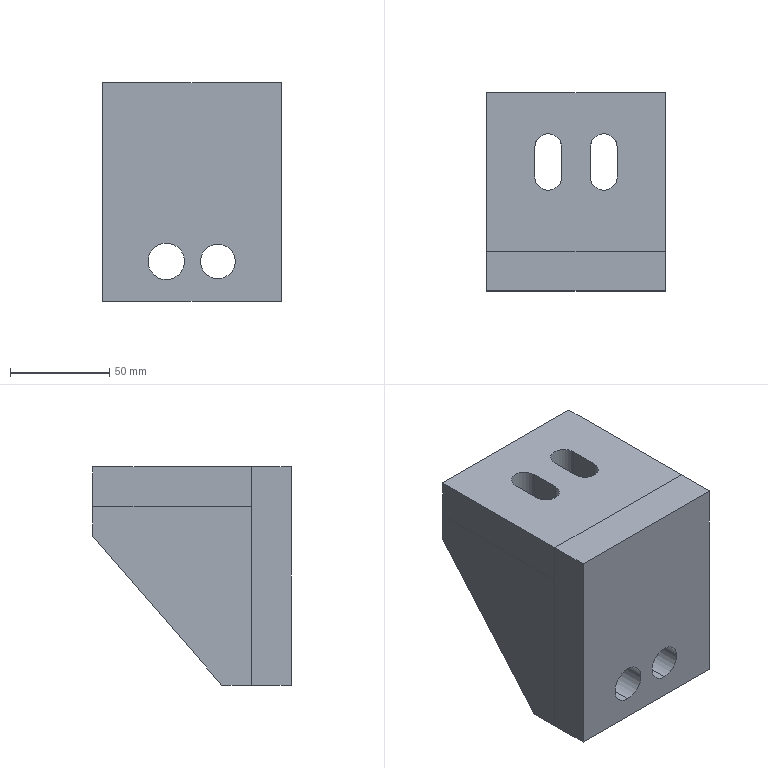Part | SolidWorks | features HoleWzd 3, ICE 2, Extrusion 1, MirrorSolid 1 | 4 solids | 38 faces | box 90 x 100 x 110 mm | volume 460863 mm3 | plane 30 | cylinder 8 | commonest cylinder face diameters 13.5 x4 17.5 x2 18.5 x2
STEP:
#1=CARTESIAN_POINT('',(-45.,20.,35.));
#2=VERTEX_POINT('',#1);
#3=CARTESIAN_POINT('',(-45.,100.,35.));
#4=VERTEX_POINT('',#3);
#5=CARTESIAN_POINT('',(-45.,100.,35.));
#6=DIRECTION('',(0.,1.,0.));
#7=VECTOR('',#6,1000.);
#8=LINE('',#5,#7);
#9=EDGE_CURVE('',#2,#4,#8,.T.);
#10=ORIENTED_EDGE('',*,*,#9,.F.);
#11=CARTESIAN_POINT('',(-30.,20.,35.));
#12=VERTEX_POINT('',#11);
#13=CARTESIAN_POINT('',(-30.,20.,35.));
#14=DIRECTION('',(-1.,0.,0.));
#15=VECTOR('',#14,1000.);
#16=LINE('',#13,#15);
#17=EDGE_CURVE('',#12,#2,#16,.T.);
#18=ORIENTED_EDGE('',*,*,#17,.F.);
#19=CARTESIAN_POINT('',(-30.,100.,35.));
#20=VERTEX_POINT('',#19);
#21=CARTESIAN_POINT('',(-30.,100.,35.));
#22=DIRECTION('',(0.,1.,0.));
#23=VECTOR('',#22,1000.);
#24=LINE('',#21,#23);
#25=EDGE_CURVE('',#12,#20,#24,.T.);
#26=ORIENTED_EDGE('',*,*,#25,.T.);
#27=CARTESIAN_POINT('',(-30.,100.,35.));
#28=DIRECTION('',(-1.,0.,0.));
#29=VECTOR('',#28,1000.);
#30=LINE('',#27,#29);
#31=EDGE_CURVE('',#20,#4,#30,.T.);
#32=ORIENTED_EDGE('',*,*,#31,.T.);
#33=EDGE_LOOP('',(#10,#18,#26,#32));
#34=FACE_OUTER_BOUND('',#33,.T.);
#35=CARTESIAN_POINT('',(-30.,100.,35.));
#36=DIRECTION('',(0.,0.,1.));
#37=DIRECTION('',(1.,0.,0.));
#38=AXIS2_PLACEMENT_3D('',#35,#36,#37);
#39=PLANE('',#38);
#40=ADVANCED_FACE('',(#34),#39,.T.);
#41=CARTESIAN_POINT('',(-45.,20.,-55.));
#42=VERTEX_POINT('',#41);
#43=CARTESIAN_POINT('',(-45.,20.,-55.));
#44=DIRECTION('',(0.,0.,1.));
#45=VECTOR('',#44,1000.);
#46=LINE('',#43,#45);
#47=EDGE_CURVE('',#42,#2,#46,.T.);
#48=ORIENTED_EDGE('',*,*,#47,.F.);
#49=CARTESIAN_POINT('',(-30.,20.,-55.));
#50=VERTEX_POINT('',#49);
#51=CARTESIAN_POINT('',(-30.,20.,-55.));
#52=DIRECTION('',(-1.,0.,0.));
#53=VECTOR('',#52,1000.);
#54=LINE('',#51,#53);
#55=EDGE_CURVE('',#50,#42,#54,.T.);
#56=ORIENTED_EDGE('',*,*,#55,.F.);
#57=CARTESIAN_POINT('',(-30.,20.,-55.));
#58=DIRECTION('',(0.,0.,1.));
#59=VECTOR('',#58,1000.);
#60=LINE('',#57,#59);
#61=EDGE_CURVE('',#50,#12,#60,.T.);
#62=ORIENTED_EDGE('',*,*,#61,.T.);
#63=ORIENTED_EDGE('',*,*,#17,.T.);
#64=EDGE_LOOP('',(#48,#56,#62,#63));
#65=FACE_OUTER_BOUND('',#64,.T.);
#66=CARTESIAN_POINT('',(-30.,20.,-55.));
#67=DIRECTION('',(0.,-1.,0.));
#68=DIRECTION('',(0.,0.,-1.));
#69=AXIS2_PLACEMENT_3D('',#66,#67,#68);
#70=PLANE('',#69);
#71=ADVANCED_FACE('',(#65),#70,.T.);
#72=CARTESIAN_POINT('',(-45.,35.,-55.));
#73=VERTEX_POINT('',#72);
#74=CARTESIAN_POINT('',(-45.,35.,-55.));
#75=DIRECTION('',(0.,-1.,0.));
#76=VECTOR('',#75,1000.);
#77=LINE('',#74,#76);
#78=EDGE_CURVE('',#73,#42,#77,.T.);
#79=ORIENTED_EDGE('',*,*,#78,.F.);
#80=CARTESIAN_POINT('',(-30.,35.,-55.));
#81=VERTEX_POINT('',#80);
#82=CARTESIAN_POINT('',(-30.,35.,-55.));
#83=DIRECTION('',(-1.,0.,0.));
#84=VECTOR('',#83,1000.);
#85=LINE('',#82,#84);
#86=EDGE_CURVE('',#81,#73,#85,.T.);
#87=ORIENTED_EDGE('',*,*,#86,.F.);
#88=CARTESIAN_POINT('',(-30.,35.,-55.));
#89=DIRECTION('',(0.,-1.,0.));
#90=VECTOR('',#89,1000.);
#91=LINE('',#88,#90);
#92=EDGE_CURVE('',#81,#50,#91,.T.);
#93=ORIENTED_EDGE('',*,*,#92,.T.);
#94=ORIENTED_EDGE('',*,*,#55,.T.);
#95=EDGE_LOOP('',(#79,#87,#93,#94));
#96=FACE_OUTER_BOUND('',#95,.T.);
#97=CARTESIAN_POINT('',(-30.,35.,-55.));
#98=DIRECTION('',(0.,0.,-1.));
#99=DIRECTION('',(-1.,0.,0.));
#100=AXIS2_PLACEMENT_3D('',#97,#98,#99);
#101=PLANE('',#100);
#102=ADVANCED_FACE('',(#96),#101,.T.);
#103=CARTESIAN_POINT('',(-45.,100.,20.));
#104=VERTEX_POINT('',#103);
#105=CARTESIAN_POINT('',(-45.,100.,20.));
#106=DIRECTION('',(0.,-0.6549,-0.7557));
#107=VECTOR('',#106,1000.);
#108=LINE('',#105,#107);
#109=EDGE_CURVE('',#104,#73,#108,.T.);
#110=ORIENTED_EDGE('',*,*,#109,.F.);
#111=CARTESIAN_POINT('',(-30.,100.,20.));
#112=VERTEX_POINT('',#111);
#113=CARTESIAN_POINT('',(-30.,100.,20.));
#114=DIRECTION('',(-1.,0.,0.));
#115=VECTOR('',#114,1000.);
#116=LINE('',#113,#115);
#117=EDGE_CURVE('',#112,#104,#116,.T.);
#118=ORIENTED_EDGE('',*,*,#117,.F.);
#119=CARTESIAN_POINT('',(-30.,100.,20.));
#120=DIRECTION('',(0.,-0.6549,-0.7557));
#121=VECTOR('',#120,1000.);
#122=LINE('',#119,#121);
#123=EDGE_CURVE('',#112,#81,#122,.T.);
#124=ORIENTED_EDGE('',*,*,#123,.T.);
#125=ORIENTED_EDGE('',*,*,#86,.T.);
#126=EDGE_LOOP('',(#110,#118,#124,#125));
#127=FACE_OUTER_BOUND('',#126,.T.);
#128=CARTESIAN_POINT('',(-30.,100.,20.));
#129=DIRECTION('',(0.,0.7557,-0.6549));
#130=DIRECTION('',(0.,0.6549,0.7557));
#131=AXIS2_PLACEMENT_3D('',#128,#129,#130);
#132=PLANE('',#131);
#133=ADVANCED_FACE('',(#127),#132,.T.);
#134=CARTESIAN_POINT('',(-45.,100.,35.));
#135=DIRECTION('',(0.,0.,-1.));
#136=VECTOR('',#135,1000.);
#137=LINE('',#134,#136);
#138=EDGE_CURVE('',#4,#104,#137,.T.);
#139=ORIENTED_EDGE('',*,*,#138,.F.);
#140=ORIENTED_EDGE('',*,*,#31,.F.);
#141=CARTESIAN_POINT('',(-30.,100.,35.));
#142=DIRECTION('',(0.,0.,-1.));
#143=VECTOR('',#142,1000.);
#144=LINE('',#141,#143);
#145=EDGE_CURVE('',#20,#112,#144,.T.);
#146=ORIENTED_EDGE('',*,*,#145,.T.);
#147=ORIENTED_EDGE('',*,*,#117,.T.);
#148=EDGE_LOOP('',(#139,#140,#146,#147));
#149=FACE_OUTER_BOUND('',#148,.T.);
#150=CARTESIAN_POINT('',(-30.,100.,35.));
#151=DIRECTION('',(0.,1.,0.));
#152=DIRECTION('',(0.,0.,1.));
#153=AXIS2_PLACEMENT_3D('',#150,#151,#152);
#154=PLANE('',#153);
#155=ADVANCED_FACE('',(#149),#154,.T.);
#156=ORIENTED_EDGE('',*,*,#25,.F.);
#157=ORIENTED_EDGE('',*,*,#61,.F.);
#158=ORIENTED_EDGE('',*,*,#92,.F.);
#159=ORIENTED_EDGE('',*,*,#123,.F.);
#160=ORIENTED_EDGE('',*,*,#145,.F.);
#161=EDGE_LOOP('',(#156,#157,#158,#159,#160));
#162=FACE_OUTER_BOUND('',#161,.T.);
#163=CARTESIAN_POINT('',(-30.,0.,0.));
#164=DIRECTION('',(-1.,0.,0.));
#165=DIRECTION('',(0.,0.,1.));
#166=AXIS2_PLACEMENT_3D('',#163,#164,#165);
#167=PLANE('',#166);
#168=ADVANCED_FACE('',(#162),#167,.F.);
#169=ORIENTED_EDGE('',*,*,#9,.T.);
#170=ORIENTED_EDGE('',*,*,#138,.T.);
#171=ORIENTED_EDGE('',*,*,#109,.T.);
#172=ORIENTED_EDGE('',*,*,#78,.T.);
#173=ORIENTED_EDGE('',*,*,#47,.T.);
#174=EDGE_LOOP('',(#169,#170,#171,#172,#173));
#175=FACE_OUTER_BOUND('',#174,.T.);
#176=CARTESIAN_POINT('',(-45.,0.,0.));
#177=DIRECTION('',(-1.,0.,0.));
#178=DIRECTION('',(0.,0.,1.));
#179=AXIS2_PLACEMENT_3D('',#176,#177,#178);
#180=PLANE('',#179);
#181=ADVANCED_FACE('',(#175),#180,.T.);
#182=CLOSED_SHELL('',(#40,#71,#102,#133,#155,#168,#181));
#183=MANIFOLD_SOLID_BREP('',#182);
#184=CARTESIAN_POINT('',(45.,20.,35.));
#185=VERTEX_POINT('',#184);
#186=CARTESIAN_POINT('',(45.,100.,35.));
#187=VERTEX_POINT('',#186);
#188=CARTESIAN_POINT('',(45.,100.,35.));
#189=DIRECTION('',(0.,1.,0.));
#190=VECTOR('',#189,1000.);
#191=LINE('',#188,#190);
#192=EDGE_CURVE('',#185,#187,#191,.T.);
#193=ORIENTED_EDGE('',*,*,#192,.T.);
#194=CARTESIAN_POINT('',(30.,100.,35.));
#195=VERTEX_POINT('',#194);
#196=CARTESIAN_POINT('',(30.,100.,35.));
#197=DIRECTION('',(1.,0.,0.));
#198=VECTOR('',#197,1000.);
#199=LINE('',#196,#198);
#200=EDGE_CURVE('',#195,#187,#199,.T.);
#201=ORIENTED_EDGE('',*,*,#200,.F.);
#202=CARTESIAN_POINT('',(30.,20.,35.));
#203=VERTEX_POINT('',#202);
#204=CARTESIAN_POINT('',(30.,100.,35.));
#205=DIRECTION('',(0.,1.,0.));
#206=VECTOR('',#205,1000.);
#207=LINE('',#204,#206);
#208=EDGE_CURVE('',#203,#195,#207,.T.);
#209=ORIENTED_EDGE('',*,*,#208,.F.);
#210=CARTESIAN_POINT('',(30.,20.,35.));
#211=DIRECTION('',(1.,0.,0.));
#212=VECTOR('',#211,1000.);
#213=LINE('',#210,#212);
#214=EDGE_CURVE('',#203,#185,#213,.T.);
#215=ORIENTED_EDGE('',*,*,#214,.T.);
#216=EDGE_LOOP('',(#193,#201,#209,#215));
#217=FACE_OUTER_BOUND('',#216,.T.);
#218=CARTESIAN_POINT('',(30.,100.,35.));
#219=DIRECTION('',(0.,0.,1.));
#220=DIRECTION('',(-1.,0.,0.));
#221=AXIS2_PLACEMENT_3D('',#218,#219,#220);
#222=PLANE('',#221);
#223=ADVANCED_FACE('',(#217),#222,.T.);
#224=CARTESIAN_POINT('',(45.,20.,-55.));
#225=VERTEX_POINT('',#224);
#226=CARTESIAN_POINT('',(45.,20.,-55.));
#227=DIRECTION('',(0.,0.,1.));
#228=VECTOR('',#227,1000.);
#229=LINE('',#226,#228);
#230=EDGE_CURVE('',#225,#185,#229,.T.);
#231=ORIENTED_EDGE('',*,*,#230,.T.);
#232=ORIENTED_EDGE('',*,*,#214,.F.);
#233=CARTESIAN_POINT('',(30.,20.,-55.));
#234=VERTEX_POINT('',#233);
#235=CARTESIAN_POINT('',(30.,20.,-55.));
#236=DIRECTION('',(0.,0.,1.));
#237=VECTOR('',#236,1000.);
#238=LINE('',#235,#237);
#239=EDGE_CURVE('',#234,#203,#238,.T.);
#240=ORIENTED_EDGE('',*,*,#239,.F.);
#241=CARTESIAN_POINT('',(30.,20.,-55.));
#242=DIRECTION('',(1.,0.,0.));
#243=VECTOR('',#242,1000.);
#244=LINE('',#241,#243);
#245=EDGE_CURVE('',#234,#225,#244,.T.);
#246=ORIENTED_EDGE('',*,*,#245,.T.);
#247=EDGE_LOOP('',(#231,#232,#240,#246));
#248=FACE_OUTER_BOUND('',#247,.T.);
#249=CARTESIAN_POINT('',(30.,20.,-55.));
#250=DIRECTION('',(0.,-1.,0.));
#251=DIRECTION('',(0.,0.,-1.));
#252=AXIS2_PLACEMENT_3D('',#249,#250,#251);
#253=PLANE('',#252);
#254=ADVANCED_FACE('',(#248),#253,.T.);
#255=CARTESIAN_POINT('',(45.,35.,-55.));
#256=VERTEX_POINT('',#255);
#257=CARTESIAN_POINT('',(45.,35.,-55.));
#258=DIRECTION('',(0.,-1.,0.));
#259=VECTOR('',#258,1000.);
#260=LINE('',#257,#259);
#261=EDGE_CURVE('',#256,#225,#260,.T.);
#262=ORIENTED_EDGE('',*,*,#261,.T.);
#263=ORIENTED_EDGE('',*,*,#245,.F.);
#264=CARTESIAN_POINT('',(30.,35.,-55.));
#265=VERTEX_POINT('',#264);
#266=CARTESIAN_POINT('',(30.,35.,-55.));
#267=DIRECTION('',(0.,-1.,0.));
#268=VECTOR('',#267,1000.);
#269=LINE('',#266,#268);
#270=EDGE_CURVE('',#265,#234,#269,.T.);
#271=ORIENTED_EDGE('',*,*,#270,.F.);
#272=CARTESIAN_POINT('',(30.,35.,-55.));
#273=DIRECTION('',(1.,0.,0.));
#274=VECTOR('',#273,1000.);
#275=LINE('',#272,#274);
#276=EDGE_CURVE('',#265,#256,#275,.T.);
#277=ORIENTED_EDGE('',*,*,#276,.T.);
#278=EDGE_LOOP('',(#262,#263,#271,#277));
#279=FACE_OUTER_BOUND('',#278,.T.);
#280=CARTESIAN_POINT('',(30.,35.,-55.));
#281=DIRECTION('',(0.,0.,-1.));
#282=DIRECTION('',(1.,0.,0.));
#283=AXIS2_PLACEMENT_3D('',#280,#281,#282);
#284=PLANE('',#283);
#285=ADVANCED_FACE('',(#279),#284,.T.);
#286=CARTESIAN_POINT('',(45.,100.,20.));
#287=VERTEX_POINT('',#286);
#288=CARTESIAN_POINT('',(45.,100.,20.));
#289=DIRECTION('',(0.,-0.6549,-0.7557));
#290=VECTOR('',#289,1000.);
#291=LINE('',#288,#290);
#292=EDGE_CURVE('',#287,#256,#291,.T.);
#293=ORIENTED_EDGE('',*,*,#292,.T.);
#294=ORIENTED_EDGE('',*,*,#276,.F.);
#295=CARTESIAN_POINT('',(30.,100.,20.));
#296=VERTEX_POINT('',#295);
#297=CARTESIAN_POINT('',(30.,100.,20.));
#298=DIRECTION('',(0.,-0.6549,-0.7557));
#299=VECTOR('',#298,1000.);
#300=LINE('',#297,#299);
#301=EDGE_CURVE('',#296,#265,#300,.T.);
#302=ORIENTED_EDGE('',*,*,#301,.F.);
#303=CARTESIAN_POINT('',(30.,100.,20.));
#304=DIRECTION('',(1.,0.,0.));
#305=VECTOR('',#304,1000.);
#306=LINE('',#303,#305);
#307=EDGE_CURVE('',#296,#287,#306,.T.);
#308=ORIENTED_EDGE('',*,*,#307,.T.);
#309=EDGE_LOOP('',(#293,#294,#302,#308));
#310=FACE_OUTER_BOUND('',#309,.T.);
#311=CARTESIAN_POINT('',(30.,100.,20.));
#312=DIRECTION('',(0.,0.7557,-0.6549));
#313=DIRECTION('',(0.,0.6549,0.7557));
#314=AXIS2_PLACEMENT_3D('',#311,#312,#313);
#315=PLANE('',#314);
#316=ADVANCED_FACE('',(#310),#315,.T.);
#317=CARTESIAN_POINT('',(45.,100.,35.));
#318=DIRECTION('',(0.,0.,-1.));
#319=VECTOR('',#318,1000.);
#320=LINE('',#317,#319);
#321=EDGE_CURVE('',#187,#287,#320,.T.);
#322=ORIENTED_EDGE('',*,*,#321,.T.);
#323=ORIENTED_EDGE('',*,*,#307,.F.);
#324=CARTESIAN_POINT('',(30.,100.,35.));
#325=DIRECTION('',(0.,0.,-1.));
#326=VECTOR('',#325,1000.);
#327=LINE('',#324,#326);
#328=EDGE_CURVE('',#195,#296,#327,.T.);
#329=ORIENTED_EDGE('',*,*,#328,.F.);
#330=ORIENTED_EDGE('',*,*,#200,.T.);
#331=EDGE_LOOP('',(#322,#323,#329,#330));
#332=FACE_OUTER_BOUND('',#331,.T.);
#333=CARTESIAN_POINT('',(30.,100.,35.));
#334=DIRECTION('',(0.,1.,0.));
#335=DIRECTION('',(0.,0.,1.));
#336=AXIS2_PLACEMENT_3D('',#333,#334,#335);
#337=PLANE('',#336);
#338=ADVANCED_FACE('',(#332),#337,.T.);
#339=ORIENTED_EDGE('',*,*,#208,.T.);
#340=ORIENTED_EDGE('',*,*,#328,.T.);
#341=ORIENTED_EDGE('',*,*,#301,.T.);
#342=ORIENTED_EDGE('',*,*,#270,.T.);
#343=ORIENTED_EDGE('',*,*,#239,.T.);
#344=EDGE_LOOP('',(#339,#340,#341,#342,#343));
#345=FACE_OUTER_BOUND('',#344,.T.);
#346=CARTESIAN_POINT('',(30.,0.,0.));
#347=DIRECTION('',(1.,0.,0.));
#348=DIRECTION('',(0.,0.,1.));
#349=AXIS2_PLACEMENT_3D('',#346,#347,#348);
#350=PLANE('',#349);
#351=ADVANCED_FACE('',(#345),#350,.F.);
#352=ORIENTED_EDGE('',*,*,#192,.F.);
#353=ORIENTED_EDGE('',*,*,#230,.F.);
#354=ORIENTED_EDGE('',*,*,#261,.F.);
#355=ORIENTED_EDGE('',*,*,#292,.F.);
#356=ORIENTED_EDGE('',*,*,#321,.F.);
#357=EDGE_LOOP('',(#352,#353,#354,#355,#356));
#358=FACE_OUTER_BOUND('',#357,.T.);
#359=CARTESIAN_POINT('',(45.,0.,0.));
#360=DIRECTION('',(1.,0.,0.));
#361=DIRECTION('',(0.,0.,1.));
#362=AXIS2_PLACEMENT_3D('',#359,#360,#361);
#363=PLANE('',#362);
#364=ADVANCED_FACE('',(#358),#363,.T.);
#365=CLOSED_SHELL('',(#223,#254,#285,#316,#338,#351,#364));
#366=MANIFOLD_SOLID_BREP('',#365);
#367=CARTESIAN_POINT('',(-45.,20.,35.));
#368=VERTEX_POINT('',#367);
#369=CARTESIAN_POINT('',(-45.,20.,55.));
#370=VERTEX_POINT('',#369);
#371=CARTESIAN_POINT('',(-45.,20.,55.));
#372=DIRECTION('',(0.,0.,1.));
#373=VECTOR('',#372,1000.);
#374=LINE('',#371,#373);
#375=EDGE_CURVE('',#368,#370,#374,.T.);
#376=ORIENTED_EDGE('',*,*,#375,.T.);
#377=CARTESIAN_POINT('',(-45.,100.,55.));
#378=VERTEX_POINT('',#377);
#379=CARTESIAN_POINT('',(-45.,100.,55.));
#380=DIRECTION('',(0.,-1.,0.));
#381=VECTOR('',#380,1000.);
#382=LINE('',#379,#381);
#383=EDGE_CURVE('',#378,#370,#382,.T.);
#384=ORIENTED_EDGE('',*,*,#383,.F.);
#385=CARTESIAN_POINT('',(-45.,100.,35.));
#386=VERTEX_POINT('',#385);
#387=CARTESIAN_POINT('',(-45.,100.,55.));
#388=DIRECTION('',(0.,0.,1.));
#389=VECTOR('',#388,1000.);
#390=LINE('',#387,#389);
#391=EDGE_CURVE('',#386,#378,#390,.T.);
#392=ORIENTED_EDGE('',*,*,#391,.F.);
#393=CARTESIAN_POINT('',(-45.,100.,35.));
#394=DIRECTION('',(0.,-1.,0.));
#395=VECTOR('',#394,1000.);
#396=LINE('',#393,#395);
#397=EDGE_CURVE('',#386,#368,#396,.T.);
#398=ORIENTED_EDGE('',*,*,#397,.T.);
#399=EDGE_LOOP('',(#376,#384,#392,#398));
#400=FACE_OUTER_BOUND('',#399,.T.);
#401=CARTESIAN_POINT('',(-45.,100.,55.));
#402=DIRECTION('',(1.,0.,0.));
#403=DIRECTION('',(0.,0.,-1.));
#404=AXIS2_PLACEMENT_3D('',#401,#402,#403);
#405=PLANE('',#404);
#406=ADVANCED_FACE('',(#400),#405,.F.);
#407=CARTESIAN_POINT('',(20.75,72.5,55.));
#408=VERTEX_POINT('',#407);
#409=CARTESIAN_POINT('',(20.75,57.5,55.));
#410=VERTEX_POINT('',#409);
#411=CARTESIAN_POINT('',(20.75,72.5,55.));
#412=DIRECTION('',(0.,-1.,0.));
#413=VECTOR('',#412,1000.);
#414=LINE('',#411,#413);
#415=EDGE_CURVE('',#408,#410,#414,.T.);
#416=ORIENTED_EDGE('',*,*,#415,.T.);
#417=CARTESIAN_POINT('',(7.25,57.5,55.));
#418=VERTEX_POINT('',#417);
#419=CARTESIAN_POINT('',(14.,57.5,55.));
#420=DIRECTION('',(0.,0.,-1.));
#421=DIRECTION('',(-1.,0.,0.));
#422=AXIS2_PLACEMENT_3D('',#419,#420,#421);
#423=CIRCLE('',#422,6.75);
#424=EDGE_CURVE('',#410,#418,#423,.T.);
#425=ORIENTED_EDGE('',*,*,#424,.T.);
#426=CARTESIAN_POINT('',(7.25,72.5,55.));
#427=VERTEX_POINT('',#426);
#428=CARTESIAN_POINT('',(7.25,72.5,55.));
#429=DIRECTION('',(0.,-1.,0.));
#430=VECTOR('',#429,1000.);
#431=LINE('',#428,#430);
#432=EDGE_CURVE('',#427,#418,#431,.T.);
#433=ORIENTED_EDGE('',*,*,#432,.F.);
#434=CARTESIAN_POINT('',(14.,72.5,55.));
#435=DIRECTION('',(0.,0.,-1.));
#436=DIRECTION('',(-1.,0.,0.));
#437=AXIS2_PLACEMENT_3D('',#434,#435,#436);
#438=CIRCLE('',#437,6.75);
#439=EDGE_CURVE('',#427,#408,#438,.T.);
#440=ORIENTED_EDGE('',*,*,#439,.T.);
#441=EDGE_LOOP('',(#416,#425,#433,#440));
#442=FACE_BOUND('',#441,.T.);
#443=CARTESIAN_POINT('',(-20.75,72.5,55.));
#444=VERTEX_POINT('',#443);
#445=CARTESIAN_POINT('',(-7.25,72.5,55.));
#446=VERTEX_POINT('',#445);
#447=CARTESIAN_POINT('',(-14.,72.5,55.));
#448=DIRECTION('',(0.,0.,-1.));
#449=DIRECTION('',(-1.,0.,0.));
#450=AXIS2_PLACEMENT_3D('',#447,#448,#449);
#451=CIRCLE('',#450,6.75);
#452=EDGE_CURVE('',#444,#446,#451,.T.);
#453=ORIENTED_EDGE('',*,*,#452,.T.);
#454=CARTESIAN_POINT('',(-7.25,57.5,55.));
#455=VERTEX_POINT('',#454);
#456=CARTESIAN_POINT('',(-7.25,72.5,55.));
#457=DIRECTION('',(0.,-1.,0.));
#458=VECTOR('',#457,1000.);
#459=LINE('',#456,#458);
#460=EDGE_CURVE('',#446,#455,#459,.T.);
#461=ORIENTED_EDGE('',*,*,#460,.T.);
#462=CARTESIAN_POINT('',(-20.75,57.5,55.));
#463=VERTEX_POINT('',#462);
#464=CARTESIAN_POINT('',(-14.,57.5,55.));
#465=DIRECTION('',(0.,0.,-1.));
#466=DIRECTION('',(-1.,0.,0.));
#467=AXIS2_PLACEMENT_3D('',#464,#465,#466);
#468=CIRCLE('',#467,6.75);
#469=EDGE_CURVE('',#455,#463,#468,.T.);
#470=ORIENTED_EDGE('',*,*,#469,.T.);
#471=CARTESIAN_POINT('',(-20.75,72.5,55.));
#472=DIRECTION('',(0.,-1.,0.));
#473=VECTOR('',#472,1000.);
#474=LINE('',#471,#473);
#475=EDGE_CURVE('',#444,#463,#474,.T.);
#476=ORIENTED_EDGE('',*,*,#475,.F.);
#477=EDGE_LOOP('',(#453,#461,#470,#476));
#478=FACE_BOUND('',#477,.T.);
#479=CARTESIAN_POINT('',(45.,20.,55.));
#480=VERTEX_POINT('',#479);
#481=CARTESIAN_POINT('',(-45.,20.,55.));
#482=DIRECTION('',(1.,0.,0.));
#483=VECTOR('',#482,1000.);
#484=LINE('',#481,#483);
#485=EDGE_CURVE('',#370,#480,#484,.T.);
#486=ORIENTED_EDGE('',*,*,#485,.T.);
#487=CARTESIAN_POINT('',(45.,100.,55.));
#488=VERTEX_POINT('',#487);
#489=CARTESIAN_POINT('',(45.,100.,55.));
#490=DIRECTION('',(0.,-1.,0.));
#491=VECTOR('',#490,1000.);
#492=LINE('',#489,#491);
#493=EDGE_CURVE('',#488,#480,#492,.T.);
#494=ORIENTED_EDGE('',*,*,#493,.F.);
#495=CARTESIAN_POINT('',(-45.,100.,55.));
#496=DIRECTION('',(1.,0.,0.));
#497=VECTOR('',#496,1000.);
#498=LINE('',#495,#497);
#499=EDGE_CURVE('',#378,#488,#498,.T.);
#500=ORIENTED_EDGE('',*,*,#499,.F.);
#501=ORIENTED_EDGE('',*,*,#383,.T.);
#502=EDGE_LOOP('',(#486,#494,#500,#501));
#503=FACE_OUTER_BOUND('',#502,.T.);
#504=CARTESIAN_POINT('',(-45.,100.,55.));
#505=DIRECTION('',(0.,0.,-1.));
#506=DIRECTION('',(-1.,0.,0.));
#507=AXIS2_PLACEMENT_3D('',#504,#505,#506);
#508=PLANE('',#507);
#509=ADVANCED_FACE('',(#442,#478,#503),#508,.F.);
#510=CARTESIAN_POINT('',(45.,20.,35.));
#511=VERTEX_POINT('',#510);
#512=CARTESIAN_POINT('',(45.,20.,55.));
#513=DIRECTION('',(0.,0.,-1.));
#514=VECTOR('',#513,1000.);
#515=LINE('',#512,#514);
#516=EDGE_CURVE('',#480,#511,#515,.T.);
#517=ORIENTED_EDGE('',*,*,#516,.T.);
#518=CARTESIAN_POINT('',(45.,100.,35.));
#519=VERTEX_POINT('',#518);
#520=CARTESIAN_POINT('',(45.,100.,35.));
#521=DIRECTION('',(0.,-1.,0.));
#522=VECTOR('',#521,1000.);
#523=LINE('',#520,#522);
#524=EDGE_CURVE('',#519,#511,#523,.T.);
#525=ORIENTED_EDGE('',*,*,#524,.F.);
#526=CARTESIAN_POINT('',(45.,100.,55.));
#527=DIRECTION('',(0.,0.,-1.));
#528=VECTOR('',#527,1000.);
#529=LINE('',#526,#528);
#530=EDGE_CURVE('',#488,#519,#529,.T.);
#531=ORIENTED_EDGE('',*,*,#530,.F.);
#532=ORIENTED_EDGE('',*,*,#493,.T.);
#533=EDGE_LOOP('',(#517,#525,#531,#532));
#534=FACE_OUTER_BOUND('',#533,.T.);
#535=CARTESIAN_POINT('',(45.,100.,55.));
#536=DIRECTION('',(-1.,0.,0.));
#537=DIRECTION('',(0.,0.,1.));
#538=AXIS2_PLACEMENT_3D('',#535,#536,#537);
#539=PLANE('',#538);
#540=ADVANCED_FACE('',(#534),#539,.F.);
#541=CARTESIAN_POINT('',(20.75,57.5,35.));
#542=VERTEX_POINT('',#541);
#543=CARTESIAN_POINT('',(7.25,57.5,35.));
#544=VERTEX_POINT('',#543);
#545=CARTESIAN_POINT('',(14.,57.5,35.));
#546=DIRECTION('',(0.,0.,-1.));
#547=DIRECTION('',(-1.,0.,0.));
#548=AXIS2_PLACEMENT_3D('',#545,#546,#547);
#549=CIRCLE('',#548,6.75);
#550=EDGE_CURVE('',#542,#544,#549,.T.);
#551=ORIENTED_EDGE('',*,*,#550,.F.);
#552=CARTESIAN_POINT('',(20.75,72.5,35.));
#553=VERTEX_POINT('',#552);
#554=CARTESIAN_POINT('',(20.75,72.5,35.));
#555=DIRECTION('',(0.,-1.,0.));
#556=VECTOR('',#555,1000.);
#557=LINE('',#554,#556);
#558=EDGE_CURVE('',#553,#542,#557,.T.);
#559=ORIENTED_EDGE('',*,*,#558,.F.);
#560=CARTESIAN_POINT('',(7.25,72.5,35.));
#561=VERTEX_POINT('',#560);
#562=CARTESIAN_POINT('',(14.,72.5,35.));
#563=DIRECTION('',(0.,0.,-1.));
#564=DIRECTION('',(-1.,0.,0.));
#565=AXIS2_PLACEMENT_3D('',#562,#563,#564);
#566=CIRCLE('',#565,6.75);
#567=EDGE_CURVE('',#561,#553,#566,.T.);
#568=ORIENTED_EDGE('',*,*,#567,.F.);
#569=CARTESIAN_POINT('',(7.25,72.5,35.));
#570=DIRECTION('',(0.,-1.,0.));
#571=VECTOR('',#570,1000.);
#572=LINE('',#569,#571);
#573=EDGE_CURVE('',#561,#544,#572,.T.);
#574=ORIENTED_EDGE('',*,*,#573,.T.);
#575=EDGE_LOOP('',(#551,#559,#568,#574));
#576=FACE_BOUND('',#575,.T.);
#577=CARTESIAN_POINT('',(-20.75,72.5,35.));
#578=VERTEX_POINT('',#577);
#579=CARTESIAN_POINT('',(-7.25,72.5,35.));
#580=VERTEX_POINT('',#579);
#581=CARTESIAN_POINT('',(-14.,72.5,35.));
#582=DIRECTION('',(0.,0.,-1.));
#583=DIRECTION('',(-1.,0.,0.));
#584=AXIS2_PLACEMENT_3D('',#581,#582,#583);
#585=CIRCLE('',#584,6.75);
#586=EDGE_CURVE('',#578,#580,#585,.T.);
#587=ORIENTED_EDGE('',*,*,#586,.F.);
#588=CARTESIAN_POINT('',(-20.75,57.5,35.));
#589=VERTEX_POINT('',#588);
#590=CARTESIAN_POINT('',(-20.75,72.5,35.));
#591=DIRECTION('',(0.,-1.,0.));
#592=VECTOR('',#591,1000.);
#593=LINE('',#590,#592);
#594=EDGE_CURVE('',#578,#589,#593,.T.);
#595=ORIENTED_EDGE('',*,*,#594,.T.);
#596=CARTESIAN_POINT('',(-7.25,57.5,35.));
#597=VERTEX_POINT('',#596);
#598=CARTESIAN_POINT('',(-14.,57.5,35.));
#599=DIRECTION('',(0.,0.,-1.));
#600=DIRECTION('',(-1.,0.,0.));
#601=AXIS2_PLACEMENT_3D('',#598,#599,#600);
#602=CIRCLE('',#601,6.75);
#603=EDGE_CURVE('',#597,#589,#602,.T.);
#604=ORIENTED_EDGE('',*,*,#603,.F.);
#605=CARTESIAN_POINT('',(-7.25,72.5,35.));
#606=DIRECTION('',(0.,-1.,0.));
#607=VECTOR('',#606,1000.);
#608=LINE('',#605,#607);
#609=EDGE_CURVE('',#580,#597,#608,.T.);
#610=ORIENTED_EDGE('',*,*,#609,.F.);
#611=EDGE_LOOP('',(#587,#595,#604,#610));
#612=FACE_BOUND('',#611,.T.);
#613=CARTESIAN_POINT('',(-45.,20.,35.));
#614=DIRECTION('',(-1.,0.,0.));
#615=VECTOR('',#614,1000.);
#616=LINE('',#613,#615);
#617=EDGE_CURVE('',#511,#368,#616,.T.);
#618=ORIENTED_EDGE('',*,*,#617,.T.);
#619=ORIENTED_EDGE('',*,*,#397,.F.);
#620=CARTESIAN_POINT('',(-45.,100.,35.));
#621=DIRECTION('',(-1.,0.,0.));
#622=VECTOR('',#621,1000.);
#623=LINE('',#620,#622);
#624=EDGE_CURVE('',#519,#386,#623,.T.);
#625=ORIENTED_EDGE('',*,*,#624,.F.);
#626=ORIENTED_EDGE('',*,*,#524,.T.);
#627=EDGE_LOOP('',(#618,#619,#625,#626));
#628=FACE_OUTER_BOUND('',#627,.T.);
#629=CARTESIAN_POINT('',(-45.,100.,35.));
#630=DIRECTION('',(0.,0.,1.));
#631=DIRECTION('',(1.,0.,0.));
#632=AXIS2_PLACEMENT_3D('',#629,#630,#631);
#633=PLANE('',#632);
#634=ADVANCED_FACE('',(#576,#612,#628),#633,.F.);
#635=ORIENTED_EDGE('',*,*,#391,.T.);
#636=ORIENTED_EDGE('',*,*,#499,.T.);
#637=ORIENTED_EDGE('',*,*,#530,.T.);
#638=ORIENTED_EDGE('',*,*,#624,.T.);
#639=EDGE_LOOP('',(#635,#636,#637,#638));
#640=FACE_OUTER_BOUND('',#639,.T.);
#641=CARTESIAN_POINT('',(0.,100.,0.));
#642=DIRECTION('',(0.,-1.,0.));
#643=DIRECTION('',(0.,0.,-1.));
#644=AXIS2_PLACEMENT_3D('',#641,#642,#643);
#645=PLANE('',#644);
#646=ADVANCED_FACE('',(#640),#645,.F.);
#647=ORIENTED_EDGE('',*,*,#375,.F.);
#648=ORIENTED_EDGE('',*,*,#617,.F.);
#649=ORIENTED_EDGE('',*,*,#516,.F.);
#650=ORIENTED_EDGE('',*,*,#485,.F.);
#651=EDGE_LOOP('',(#647,#648,#649,#650));
#652=FACE_OUTER_BOUND('',#651,.T.);
#653=CARTESIAN_POINT('',(0.,20.,0.));
#654=DIRECTION('',(0.,-1.,0.));
#655=DIRECTION('',(0.,0.,-1.));
#656=AXIS2_PLACEMENT_3D('',#653,#654,#655);
#657=PLANE('',#656);
#658=ADVANCED_FACE('',(#652),#657,.T.);
#659=ORIENTED_EDGE('',*,*,#469,.F.);
#660=CARTESIAN_POINT('',(-7.25,57.5,55.));
#661=DIRECTION('',(0.,0.,1.));
#662=VECTOR('',#661,1000.);
#663=LINE('',#660,#662);
#664=EDGE_CURVE('',#597,#455,#663,.T.);
#665=ORIENTED_EDGE('',*,*,#664,.F.);
#666=ORIENTED_EDGE('',*,*,#603,.T.);
#667=CARTESIAN_POINT('',(-20.75,57.5,35.));
#668=DIRECTION('',(0.,0.,-1.));
#669=VECTOR('',#668,1000.);
#670=LINE('',#667,#669);
#671=EDGE_CURVE('',#463,#589,#670,.T.);
#672=ORIENTED_EDGE('',*,*,#671,.F.);
#673=EDGE_LOOP('',(#659,#665,#666,#672));
#674=FACE_OUTER_BOUND('',#673,.T.);
#675=CARTESIAN_POINT('',(-14.,57.5,35.));
#676=DIRECTION('',(0.,0.,-1.));
#677=DIRECTION('',(-1.,0.,0.));
#678=AXIS2_PLACEMENT_3D('',#675,#676,#677);
#679=CYLINDRICAL_SURFACE('',#678,6.75);
#680=ADVANCED_FACE('',(#674),#679,.F.);
#681=ORIENTED_EDGE('',*,*,#586,.T.);
#682=CARTESIAN_POINT('',(-7.25,72.5,55.));
#683=DIRECTION('',(0.,0.,1.));
#684=VECTOR('',#683,1000.);
#685=LINE('',#682,#684);
#686=EDGE_CURVE('',#580,#446,#685,.T.);
#687=ORIENTED_EDGE('',*,*,#686,.T.);
#688=ORIENTED_EDGE('',*,*,#452,.F.);
#689=CARTESIAN_POINT('',(-20.75,72.5,35.));
#690=DIRECTION('',(0.,0.,1.));
#691=VECTOR('',#690,1000.);
#692=LINE('',#689,#691);
#693=EDGE_CURVE('',#578,#444,#692,.T.);
#694=ORIENTED_EDGE('',*,*,#693,.F.);
#695=EDGE_LOOP('',(#681,#687,#688,#694));
#696=FACE_OUTER_BOUND('',#695,.T.);
#697=CARTESIAN_POINT('',(-14.,72.5,35.));
#698=DIRECTION('',(0.,0.,-1.));
#699=DIRECTION('',(-1.,0.,0.));
#700=AXIS2_PLACEMENT_3D('',#697,#698,#699);
#701=CYLINDRICAL_SURFACE('',#700,6.75);
#702=ADVANCED_FACE('',(#696),#701,.F.);
#703=ORIENTED_EDGE('',*,*,#671,.T.);
#704=ORIENTED_EDGE('',*,*,#594,.F.);
#705=ORIENTED_EDGE('',*,*,#693,.T.);
#706=ORIENTED_EDGE('',*,*,#475,.T.);
#707=EDGE_LOOP('',(#703,#704,#705,#706));
#708=FACE_OUTER_BOUND('',#707,.T.);
#709=CARTESIAN_POINT('',(-20.75,72.5,35.));
#710=DIRECTION('',(-1.,0.,0.));
#711=DIRECTION('',(0.,0.,1.));
#712=AXIS2_PLACEMENT_3D('',#709,#710,#711);
#713=PLANE('',#712);
#714=ADVANCED_FACE('',(#708),#713,.F.);
#715=ORIENTED_EDGE('',*,*,#664,.T.);
#716=ORIENTED_EDGE('',*,*,#460,.F.);
#717=ORIENTED_EDGE('',*,*,#686,.F.);
#718=ORIENTED_EDGE('',*,*,#609,.T.);
#719=EDGE_LOOP('',(#715,#716,#717,#718));
#720=FACE_OUTER_BOUND('',#719,.T.);
#721=CARTESIAN_POINT('',(-7.25,72.5,55.));
#722=DIRECTION('',(1.,0.,0.));
#723=DIRECTION('',(0.,0.,-1.));
#724=AXIS2_PLACEMENT_3D('',#721,#722,#723);
#725=PLANE('',#724);
#726=ADVANCED_FACE('',(#720),#725,.F.);
#727=ORIENTED_EDGE('',*,*,#424,.F.);
#728=CARTESIAN_POINT('',(20.75,57.5,55.));
#729=DIRECTION('',(0.,0.,1.));
#730=VECTOR('',#729,1000.);
#731=LINE('',#728,#730);
#732=EDGE_CURVE('',#542,#410,#731,.T.);
#733=ORIENTED_EDGE('',*,*,#732,.F.);
#734=ORIENTED_EDGE('',*,*,#550,.T.);
#735=CARTESIAN_POINT('',(7.25,57.5,35.));
#736=DIRECTION('',(0.,0.,-1.));
#737=VECTOR('',#736,1000.);
#738=LINE('',#735,#737);
#739=EDGE_CURVE('',#418,#544,#738,.T.);
#740=ORIENTED_EDGE('',*,*,#739,.F.);
#741=EDGE_LOOP('',(#727,#733,#734,#740));
#742=FACE_OUTER_BOUND('',#741,.T.);
#743=CARTESIAN_POINT('',(14.,57.5,35.));
#744=DIRECTION('',(0.,0.,-1.));
#745=DIRECTION('',(-1.,0.,0.));
#746=AXIS2_PLACEMENT_3D('',#743,#744,#745);
#747=CYLINDRICAL_SURFACE('',#746,6.75);
#748=ADVANCED_FACE('',(#742),#747,.F.);
#749=ORIENTED_EDGE('',*,*,#567,.T.);
#750=CARTESIAN_POINT('',(20.75,72.5,55.));
#751=DIRECTION('',(0.,0.,1.));
#752=VECTOR('',#751,1000.);
#753=LINE('',#750,#752);
#754=EDGE_CURVE('',#553,#408,#753,.T.);
#755=ORIENTED_EDGE('',*,*,#754,.T.);
#756=ORIENTED_EDGE('',*,*,#439,.F.);
#757=CARTESIAN_POINT('',(7.25,72.5,35.));
#758=DIRECTION('',(0.,0.,1.));
#759=VECTOR('',#758,1000.);
#760=LINE('',#757,#759);
#761=EDGE_CURVE('',#561,#427,#760,.T.);
#762=ORIENTED_EDGE('',*,*,#761,.F.);
#763=EDGE_LOOP('',(#749,#755,#756,#762));
#764=FACE_OUTER_BOUND('',#763,.T.);
#765=CARTESIAN_POINT('',(14.,72.5,35.));
#766=DIRECTION('',(0.,0.,-1.));
#767=DIRECTION('',(-1.,0.,0.));
#768=AXIS2_PLACEMENT_3D('',#765,#766,#767);
#769=CYLINDRICAL_SURFACE('',#768,6.75);
#770=ADVANCED_FACE('',(#764),#769,.F.);
#771=ORIENTED_EDGE('',*,*,#739,.T.);
#772=ORIENTED_EDGE('',*,*,#573,.F.);
#773=ORIENTED_EDGE('',*,*,#761,.T.);
#774=ORIENTED_EDGE('',*,*,#432,.T.);
#775=EDGE_LOOP('',(#771,#772,#773,#774));
#776=FACE_OUTER_BOUND('',#775,.T.);
#777=CARTESIAN_POINT('',(7.25,72.5,35.));
#778=DIRECTION('',(-1.,0.,0.));
#779=DIRECTION('',(0.,0.,1.));
#780=AXIS2_PLACEMENT_3D('',#777,#778,#779);
#781=PLANE('',#780);
#782=ADVANCED_FACE('',(#776),#781,.F.);
#783=ORIENTED_EDGE('',*,*,#732,.T.);
#784=ORIENTED_EDGE('',*,*,#415,.F.);
#785=ORIENTED_EDGE('',*,*,#754,.F.);
#786=ORIENTED_EDGE('',*,*,#558,.T.);
#787=EDGE_LOOP('',(#783,#784,#785,#786));
#788=FACE_OUTER_BOUND('',#787,.T.);
#789=CARTESIAN_POINT('',(20.75,72.5,55.));
#790=DIRECTION('',(1.,0.,0.));
#791=DIRECTION('',(0.,0.,-1.));
#792=AXIS2_PLACEMENT_3D('',#789,#790,#791);
#793=PLANE('',#792);
#794=ADVANCED_FACE('',(#788),#793,.F.);
#795=CLOSED_SHELL('',(#406,#509,#540,#634,#646,#658,#680,#702,#714,#726,#748,#770,#782,#794));
#796=MANIFOLD_SOLID_BREP('',#795);
#797=CARTESIAN_POINT('',(13.,0.,-43.75));
#798=VERTEX_POINT('',#797);
#799=CARTESIAN_POINT('',(13.,0.,-26.25));
#800=VERTEX_POINT('',#799);
#801=CARTESIAN_POINT('',(13.,0.,-35.));
#802=DIRECTION('',(0.,1.,0.));
#803=DIRECTION('',(0.,0.,1.));
#804=AXIS2_PLACEMENT_3D('',#801,#802,#803);
#805=CIRCLE('',#804,8.75);
#806=EDGE_CURVE('',#798,#800,#805,.T.);
#807=ORIENTED_EDGE('',*,*,#806,.F.);
#808=CARTESIAN_POINT('',(13.,20.,-43.75));
#809=VERTEX_POINT('',#808);
#810=CARTESIAN_POINT('',(13.,20.,-43.75));
#811=DIRECTION('',(0.,1.,0.));
#812=VECTOR('',#811,1000.);
#813=LINE('',#810,#812);
#814=EDGE_CURVE('',#798,#809,#813,.T.);
#815=ORIENTED_EDGE('',*,*,#814,.T.);
#816=CARTESIAN_POINT('',(13.,20.,-26.25));
#817=VERTEX_POINT('',#816);
#818=CARTESIAN_POINT('',(13.,20.,-35.));
#819=DIRECTION('',(0.,1.,0.));
#820=DIRECTION('',(0.,0.,1.));
#821=AXIS2_PLACEMENT_3D('',#818,#819,#820);
#822=CIRCLE('',#821,8.75);
#823=EDGE_CURVE('',#809,#817,#822,.T.);
#824=ORIENTED_EDGE('',*,*,#823,.T.);
#825=CARTESIAN_POINT('',(13.,20.,-26.25));
#826=DIRECTION('',(0.,1.,0.));
#827=VECTOR('',#826,1000.);
#828=LINE('',#825,#827);
#829=EDGE_CURVE('',#800,#817,#828,.T.);
#830=ORIENTED_EDGE('',*,*,#829,.F.);
#831=EDGE_LOOP('',(#807,#815,#824,#830));
#832=FACE_OUTER_BOUND('',#831,.T.);
#833=CARTESIAN_POINT('',(13.,20.,-35.));
#834=DIRECTION('',(0.,1.,0.));
#835=DIRECTION('',(0.,0.,1.));
#836=AXIS2_PLACEMENT_3D('',#833,#834,#835);
#837=CYLINDRICAL_SURFACE('',#836,8.75);
#838=ADVANCED_FACE('',(#832),#837,.F.);
#839=CARTESIAN_POINT('',(-13.,0.,-44.25));
#840=VERTEX_POINT('',#839);
#841=CARTESIAN_POINT('',(-13.,0.,-25.75));
#842=VERTEX_POINT('',#841);
#843=CARTESIAN_POINT('',(-13.,0.,-35.));
#844=DIRECTION('',(0.,1.,0.));
#845=DIRECTION('',(0.,0.,1.));
#846=AXIS2_PLACEMENT_3D('',#843,#844,#845);
#847=CIRCLE('',#846,9.25);
#848=EDGE_CURVE('',#840,#842,#847,.T.);
#849=ORIENTED_EDGE('',*,*,#848,.F.);
#850=CARTESIAN_POINT('',(-13.,20.,-44.25));
#851=VERTEX_POINT('',#850);
#852=CARTESIAN_POINT('',(-13.,20.,-44.25));
#853=DIRECTION('',(0.,1.,0.));
#854=VECTOR('',#853,1000.);
#855=LINE('',#852,#854);
#856=EDGE_CURVE('',#840,#851,#855,.T.);
#857=ORIENTED_EDGE('',*,*,#856,.T.);
#858=CARTESIAN_POINT('',(-13.,20.,-25.75));
#859=VERTEX_POINT('',#858);
#860=CARTESIAN_POINT('',(-13.,20.,-35.));
#861=DIRECTION('',(0.,1.,0.));
#862=DIRECTION('',(0.,0.,1.));
#863=AXIS2_PLACEMENT_3D('',#860,#861,#862);
#864=CIRCLE('',#863,9.25);
#865=EDGE_CURVE('',#851,#859,#864,.T.);
#866=ORIENTED_EDGE('',*,*,#865,.T.);
#867=CARTESIAN_POINT('',(-13.,20.,-25.75));
#868=DIRECTION('',(0.,1.,0.));
#869=VECTOR('',#868,1000.);
#870=LINE('',#867,#869);
#871=EDGE_CURVE('',#842,#859,#870,.T.);
#872=ORIENTED_EDGE('',*,*,#871,.F.);
#873=EDGE_LOOP('',(#849,#857,#866,#872));
#874=FACE_OUTER_BOUND('',#873,.T.);
#875=CARTESIAN_POINT('',(-13.,20.,-35.));
#876=DIRECTION('',(0.,1.,0.));
#877=DIRECTION('',(0.,0.,1.));
#878=AXIS2_PLACEMENT_3D('',#875,#876,#877);
#879=CYLINDRICAL_SURFACE('',#878,9.25);
#880=ADVANCED_FACE('',(#874),#879,.F.);
#881=CARTESIAN_POINT('',(45.,0.,55.));
#882=VERTEX_POINT('',#881);
#883=CARTESIAN_POINT('',(45.,0.,-55.));
#884=VERTEX_POINT('',#883);
#885=CARTESIAN_POINT('',(45.,0.,55.));
#886=DIRECTION('',(0.,0.,-1.));
#887=VECTOR('',#886,1000.);
#888=LINE('',#885,#887);
#889=EDGE_CURVE('',#882,#884,#888,.T.);
#890=ORIENTED_EDGE('',*,*,#889,.T.);
#891=CARTESIAN_POINT('',(45.,20.,-55.));
#892=VERTEX_POINT('',#891);
#893=CARTESIAN_POINT('',(45.,20.,-55.));
#894=DIRECTION('',(0.,-1.,0.));
#895=VECTOR('',#894,1000.);
#896=LINE('',#893,#895);
#897=EDGE_CURVE('',#892,#884,#896,.T.);
#898=ORIENTED_EDGE('',*,*,#897,.F.);
#899=CARTESIAN_POINT('',(45.,20.,55.));
#900=VERTEX_POINT('',#899);
#901=CARTESIAN_POINT('',(45.,20.,55.));
#902=DIRECTION('',(0.,0.,-1.));
#903=VECTOR('',#902,1000.);
#904=LINE('',#901,#903);
#905=EDGE_CURVE('',#900,#892,#904,.T.);
#906=ORIENTED_EDGE('',*,*,#905,.F.);
#907=CARTESIAN_POINT('',(45.,20.,55.));
#908=DIRECTION('',(0.,-1.,0.));
#909=VECTOR('',#908,1000.);
#910=LINE('',#907,#909);
#911=EDGE_CURVE('',#900,#882,#910,.T.);
#912=ORIENTED_EDGE('',*,*,#911,.T.);
#913=EDGE_LOOP('',(#890,#898,#906,#912));
#914=FACE_OUTER_BOUND('',#913,.T.);
#915=CARTESIAN_POINT('',(45.,20.,55.));
#916=DIRECTION('',(-1.,0.,0.));
#917=DIRECTION('',(0.,0.,1.));
#918=AXIS2_PLACEMENT_3D('',#915,#916,#917);
#919=PLANE('',#918);
#920=ADVANCED_FACE('',(#914),#919,.F.);
#921=CARTESIAN_POINT('',(-45.,0.,-55.));
#922=VERTEX_POINT('',#921);
#923=CARTESIAN_POINT('',(-45.,0.,-55.));
#924=DIRECTION('',(-1.,0.,0.));
#925=VECTOR('',#924,1000.);
#926=LINE('',#923,#925);
#927=EDGE_CURVE('',#884,#922,#926,.T.);
#928=ORIENTED_EDGE('',*,*,#927,.T.);
#929=CARTESIAN_POINT('',(-45.,20.,-55.));
#930=VERTEX_POINT('',#929);
#931=CARTESIAN_POINT('',(-45.,20.,-55.));
#932=DIRECTION('',(0.,-1.,0.));
#933=VECTOR('',#932,1000.);
#934=LINE('',#931,#933);
#935=EDGE_CURVE('',#930,#922,#934,.T.);
#936=ORIENTED_EDGE('',*,*,#935,.F.);
#937=CARTESIAN_POINT('',(-45.,20.,-55.));
#938=DIRECTION('',(-1.,0.,0.));
#939=VECTOR('',#938,1000.);
#940=LINE('',#937,#939);
#941=EDGE_CURVE('',#892,#930,#940,.T.);
#942=ORIENTED_EDGE('',*,*,#941,.F.);
#943=ORIENTED_EDGE('',*,*,#897,.T.);
#944=EDGE_LOOP('',(#928,#936,#942,#943));
#945=FACE_OUTER_BOUND('',#944,.T.);
#946=CARTESIAN_POINT('',(-45.,20.,-55.));
#947=DIRECTION('',(0.,0.,1.));
#948=DIRECTION('',(1.,0.,0.));
#949=AXIS2_PLACEMENT_3D('',#946,#947,#948);
#950=PLANE('',#949);
#951=ADVANCED_FACE('',(#945),#950,.F.);
#952=CARTESIAN_POINT('',(-45.,0.,55.));
#953=VERTEX_POINT('',#952);
#954=CARTESIAN_POINT('',(-45.,0.,55.));
#955=DIRECTION('',(0.,0.,1.));
#956=VECTOR('',#955,1000.);
#957=LINE('',#954,#956);
#958=EDGE_CURVE('',#922,#953,#957,.T.);
#959=ORIENTED_EDGE('',*,*,#958,.T.);
#960=CARTESIAN_POINT('',(-45.,20.,55.));
#961=VERTEX_POINT('',#960);
#962=CARTESIAN_POINT('',(-45.,20.,55.));
#963=DIRECTION('',(0.,-1.,0.));
#964=VECTOR('',#963,1000.);
#965=LINE('',#962,#964);
#966=EDGE_CURVE('',#961,#953,#965,.T.);
#967=ORIENTED_EDGE('',*,*,#966,.F.);
#968=CARTESIAN_POINT('',(-45.,20.,55.));
#969=DIRECTION('',(0.,0.,1.));
#970=VECTOR('',#969,1000.);
#971=LINE('',#968,#970);
#972=EDGE_CURVE('',#930,#961,#971,.T.);
#973=ORIENTED_EDGE('',*,*,#972,.F.);
#974=ORIENTED_EDGE('',*,*,#935,.T.);
#975=EDGE_LOOP('',(#959,#967,#973,#974));
#976=FACE_OUTER_BOUND('',#975,.T.);
#977=CARTESIAN_POINT('',(-45.,20.,55.));
#978=DIRECTION('',(1.,0.,0.));
#979=DIRECTION('',(0.,0.,-1.));
#980=AXIS2_PLACEMENT_3D('',#977,#978,#979);
#981=PLANE('',#980);
#982=ADVANCED_FACE('',(#976),#981,.F.);
#983=CARTESIAN_POINT('',(-45.,0.,55.));
#984=DIRECTION('',(1.,0.,0.));
#985=VECTOR('',#984,1000.);
#986=LINE('',#983,#985);
#987=EDGE_CURVE('',#953,#882,#986,.T.);
#988=ORIENTED_EDGE('',*,*,#987,.T.);
#989=ORIENTED_EDGE('',*,*,#911,.F.);
#990=CARTESIAN_POINT('',(-45.,20.,55.));
#991=DIRECTION('',(1.,0.,0.));
#992=VECTOR('',#991,1000.);
#993=LINE('',#990,#992);
#994=EDGE_CURVE('',#961,#900,#993,.T.);
#995=ORIENTED_EDGE('',*,*,#994,.F.);
#996=ORIENTED_EDGE('',*,*,#966,.T.);
#997=EDGE_LOOP('',(#988,#989,#995,#996));
#998=FACE_OUTER_BOUND('',#997,.T.);
#999=CARTESIAN_POINT('',(-45.,20.,55.));
#1000=DIRECTION('',(0.,0.,-1.));
#1001=DIRECTION('',(-1.,0.,0.));
#1002=AXIS2_PLACEMENT_3D('',#999,#1000,#1001);
#1003=PLANE('',#1002);
#1004=ADVANCED_FACE('',(#998),#1003,.F.);
#1005=CARTESIAN_POINT('',(13.,20.,-35.));
#1006=DIRECTION('',(0.,1.,0.));
#1007=DIRECTION('',(0.,0.,1.));
#1008=AXIS2_PLACEMENT_3D('',#1005,#1006,#1007);
#1009=CIRCLE('',#1008,8.75);
#1010=EDGE_CURVE('',#817,#809,#1009,.T.);
#1011=ORIENTED_EDGE('',*,*,#1010,.F.);
#1012=ORIENTED_EDGE('',*,*,#823,.F.);
#1013=EDGE_LOOP('',(#1011,#1012));
#1014=FACE_BOUND('',#1013,.T.);
#1015=CARTESIAN_POINT('',(-13.,20.,-35.));
#1016=DIRECTION('',(0.,1.,0.));
#1017=DIRECTION('',(0.,0.,1.));
#1018=AXIS2_PLACEMENT_3D('',#1015,#1016,#1017);
#1019=CIRCLE('',#1018,9.25);
#1020=EDGE_CURVE('',#859,#851,#1019,.T.);
#1021=ORIENTED_EDGE('',*,*,#1020,.F.);
#1022=ORIENTED_EDGE('',*,*,#865,.F.);
#1023=EDGE_LOOP('',(#1021,#1022));
#1024=FACE_BOUND('',#1023,.T.);
#1025=ORIENTED_EDGE('',*,*,#905,.T.);
#1026=ORIENTED_EDGE('',*,*,#941,.T.);
#1027=ORIENTED_EDGE('',*,*,#972,.T.);
#1028=ORIENTED_EDGE('',*,*,#994,.T.);
#1029=EDGE_LOOP('',(#1025,#1026,#1027,#1028));
#1030=FACE_OUTER_BOUND('',#1029,.T.);
#1031=CARTESIAN_POINT('',(0.,20.,0.));
#1032=DIRECTION('',(0.,-1.,0.));
#1033=DIRECTION('',(0.,0.,-1.));
#1034=AXIS2_PLACEMENT_3D('',#1031,#1032,#1033);
#1035=PLANE('',#1034);
#1036=ADVANCED_FACE('',(#1014,#1024,#1030),#1035,.F.);
#1037=CARTESIAN_POINT('',(13.,0.,-35.));
#1038=DIRECTION('',(0.,1.,0.));
#1039=DIRECTION('',(0.,0.,1.));
#1040=AXIS2_PLACEMENT_3D('',#1037,#1038,#1039);
#1041=CIRCLE('',#1040,8.75);
#1042=EDGE_CURVE('',#800,#798,#1041,.T.);
#1043=ORIENTED_EDGE('',*,*,#1042,.T.);
#1044=ORIENTED_EDGE('',*,*,#806,.T.);
#1045=EDGE_LOOP('',(#1043,#1044));
#1046=FACE_BOUND('',#1045,.T.);
#1047=CARTESIAN_POINT('',(-13.,0.,-35.));
#1048=DIRECTION('',(0.,1.,0.));
#1049=DIRECTION('',(0.,0.,1.));
#1050=AXIS2_PLACEMENT_3D('',#1047,#1048,#1049);
#1051=CIRCLE('',#1050,9.25);
#1052=EDGE_CURVE('',#842,#840,#1051,.T.);
#1053=ORIENTED_EDGE('',*,*,#1052,.T.);
#1054=ORIENTED_EDGE('',*,*,#848,.T.);
#1055=EDGE_LOOP('',(#1053,#1054));
#1056=FACE_BOUND('',#1055,.T.);
#1057=ORIENTED_EDGE('',*,*,#889,.F.);
#1058=ORIENTED_EDGE('',*,*,#987,.F.);
#1059=ORIENTED_EDGE('',*,*,#958,.F.);
#1060=ORIENTED_EDGE('',*,*,#927,.F.);
#1061=EDGE_LOOP('',(#1057,#1058,#1059,#1060));
#1062=FACE_OUTER_BOUND('',#1061,.T.);
#1063=CARTESIAN_POINT('',(0.,0.,0.));
#1064=DIRECTION('',(0.,-1.,0.));
#1065=DIRECTION('',(0.,0.,-1.));
#1066=AXIS2_PLACEMENT_3D('',#1063,#1064,#1065);
#1067=PLANE('',#1066);
#1068=ADVANCED_FACE('',(#1046,#1056,#1062),#1067,.T.);
#1069=ORIENTED_EDGE('',*,*,#856,.F.);
#1070=ORIENTED_EDGE('',*,*,#1052,.F.);
#1071=ORIENTED_EDGE('',*,*,#871,.T.);
#1072=ORIENTED_EDGE('',*,*,#1020,.T.);
#1073=EDGE_LOOP('',(#1069,#1070,#1071,#1072));
#1074=FACE_OUTER_BOUND('',#1073,.T.);
#1075=CARTESIAN_POINT('',(-13.,20.,-35.));
#1076=DIRECTION('',(0.,1.,0.));
#1077=DIRECTION('',(0.,0.,1.));
#1078=AXIS2_PLACEMENT_3D('',#1075,#1076,#1077);
#1079=CYLINDRICAL_SURFACE('',#1078,9.25);
#1080=ADVANCED_FACE('',(#1074),#1079,.F.);
#1081=ORIENTED_EDGE('',*,*,#814,.F.);
#1082=ORIENTED_EDGE('',*,*,#1042,.F.);
#1083=ORIENTED_EDGE('',*,*,#829,.T.);
#1084=ORIENTED_EDGE('',*,*,#1010,.T.);
#1085=EDGE_LOOP('',(#1081,#1082,#1083,#1084));
#1086=FACE_OUTER_BOUND('',#1085,.T.);
#1087=CARTESIAN_POINT('',(13.,20.,-35.));
#1088=DIRECTION('',(0.,1.,0.));
#1089=DIRECTION('',(0.,0.,1.));
#1090=AXIS2_PLACEMENT_3D('',#1087,#1088,#1089);
#1091=CYLINDRICAL_SURFACE('',#1090,8.75);
#1092=ADVANCED_FACE('',(#1086),#1091,.F.);
#1093=CLOSED_SHELL('',(#838,#880,#920,#951,#982,#1004,#1036,#1068,#1080,#1092));
#1094=MANIFOLD_SOLID_BREP('',#1093);
#1095=CARTESIAN_POINT('',(0.,0.,0.));
#1096=DIRECTION('',(0.,0.,1.));
#1097=DIRECTION('',(1.,0.,0.));
#1098=AXIS2_PLACEMENT_3D('',#1095,#1096,#1097);
#1099=(LENGTH_UNIT()NAMED_UNIT(*)SI_UNIT(.MILLI.,.METRE.));
#1100=UNCERTAINTY_MEASURE_WITH_UNIT(LENGTH_MEASURE(0.00001),#1099,'','');
#1101=(NAMED_UNIT(*)PLANE_ANGLE_UNIT()SI_UNIT($,.RADIAN.));
#1102=(NAMED_UNIT(*)SI_UNIT($,.STERADIAN.)SOLID_ANGLE_UNIT());
#1103=(GEOMETRIC_REPRESENTATION_CONTEXT(3)GLOBAL_UNCERTAINTY_ASSIGNED_CONTEXT((#1100))GLOBAL_UNIT_ASSIGNED_CONTEXT((#1099,#1101,#1102))REPRESENTATION_CONTEXT('',''));
#1104=ADVANCED_BREP_SHAPE_REPRESENTATION('',(#183,#366,#796,#1094,#1098),#1103);